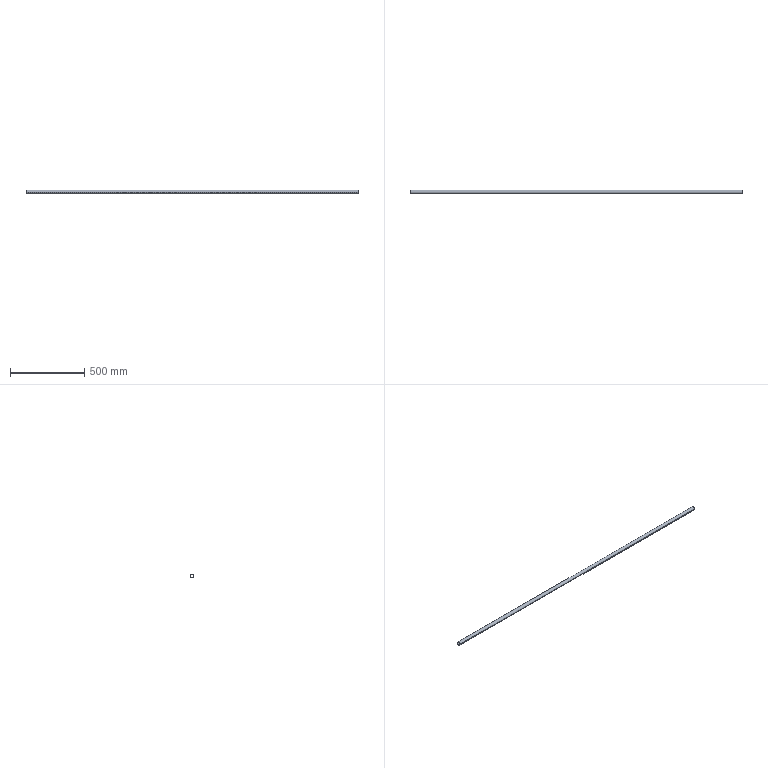Part | STEP file | 电柜通道护栏1栏杆_Default<As Machined> | 1 solid | 6 faces | box 2240 x 25 x 25 mm | volume 248060 mm3 | cylinder 4 | plane 2 | commonest cylinder face diameters 22 x2 25 x2
STEP:
#1=CARTESIAN_POINT('',(0.,0.,0.));
#2=DIRECTION('',(0.,0.,1.));
#3=DIRECTION('',(1.,0.,0.));
#4=AXIS2_PLACEMENT_3D('',#1,#2,#3);
#5=CARTESIAN_POINT('',(1120.,12.5,0.));
#6=VERTEX_POINT('',#5);
#7=CARTESIAN_POINT('',(1120.,-12.5,0.));
#8=VERTEX_POINT('',#7);
#9=CARTESIAN_POINT('',(1120.,0.,0.));
#10=DIRECTION('',(1.,0.,0.));
#11=DIRECTION('',(0.,1.,0.));
#12=AXIS2_PLACEMENT_3D('',#9,#10,#11);
#13=CIRCLE('',#12,12.5);
#14=CARTESIAN_POINT('',(1120.,0.,0.));
#15=DIRECTION('',(-1.,0.,0.));
#16=DIRECTION('',(0.,-1.,0.));
#17=AXIS2_PLACEMENT_3D('',#14,#15,#16);
#18=CYLINDRICAL_SURFACE('',#17,12.5);
#19=CARTESIAN_POINT('',(3.142,0.));
#20=DIRECTION('',(-1.,0.));
#21=VECTOR('',#20,1.);
#22=LINE('',#19,#21);
#23=(GEOMETRIC_REPRESENTATION_CONTEXT(2)PARAMETRIC_REPRESENTATION_CONTEXT()REPRESENTATION_CONTEXT('',''));
#24=DEFINITIONAL_REPRESENTATION('',(#22),#23);
#25=PCURVE('',#18,#24);
#26=CARTESIAN_POINT('',(1120.,0.,0.));
#27=DIRECTION('',(1.,0.,0.));
#28=DIRECTION('',(0.,1.,0.));
#29=AXIS2_PLACEMENT_3D('',#26,#27,#28);
#30=PLANE('',#29);
#31=CARTESIAN_POINT('',(0.,0.));
#32=DIRECTION('',(1.,0.));
#33=AXIS2_PLACEMENT_2D('',#31,#32);
#34=CIRCLE('',#33,12.5);
#35=(GEOMETRIC_REPRESENTATION_CONTEXT(2)PARAMETRIC_REPRESENTATION_CONTEXT()REPRESENTATION_CONTEXT('',''));
#36=DEFINITIONAL_REPRESENTATION('',(#34),#35);
#37=PCURVE('',#30,#36);
#38=SURFACE_CURVE('',#13,(#25,#37),.PCURVE_S1.);
#39=EDGE_CURVE('',#6,#8,#38,.T.);
#40=ORIENTED_EDGE('',*,*,#39,.F.);
#41=CARTESIAN_POINT('',(-1120.,12.5,0.));
#42=VERTEX_POINT('',#41);
#43=CARTESIAN_POINT('',(1120.,12.5,0.));
#44=DIRECTION('',(-1.,0.,0.));
#45=VECTOR('',#44,1.);
#46=LINE('',#43,#45);
#47=CARTESIAN_POINT('',(3.142,0.));
#48=DIRECTION('',(0.,1.));
#49=VECTOR('',#48,1.);
#50=LINE('',#47,#49);
#51=(GEOMETRIC_REPRESENTATION_CONTEXT(2)PARAMETRIC_REPRESENTATION_CONTEXT()REPRESENTATION_CONTEXT('',''));
#52=DEFINITIONAL_REPRESENTATION('',(#50),#51);
#53=PCURVE('',#18,#52);
#54=CARTESIAN_POINT('',(1120.,0.,0.));
#55=DIRECTION('',(-1.,0.,0.));
#56=DIRECTION('',(0.,-1.,0.));
#57=AXIS2_PLACEMENT_3D('',#54,#55,#56);
#58=CYLINDRICAL_SURFACE('',#57,12.5);
#59=CARTESIAN_POINT('',(3.142,0.));
#60=DIRECTION('',(0.,1.));
#61=VECTOR('',#60,1.);
#62=LINE('',#59,#61);
#63=(GEOMETRIC_REPRESENTATION_CONTEXT(2)PARAMETRIC_REPRESENTATION_CONTEXT()REPRESENTATION_CONTEXT('',''));
#64=DEFINITIONAL_REPRESENTATION('',(#62),#63);
#65=PCURVE('',#58,#64);
#66=SURFACE_CURVE('',#46,(#53,#65),.PCURVE_S1.);
#67=EDGE_CURVE('',#6,#42,#66,.T.);
#68=ORIENTED_EDGE('',*,*,#67,.T.);
#69=CARTESIAN_POINT('',(-1120.,-12.5,0.));
#70=VERTEX_POINT('',#69);
#71=CARTESIAN_POINT('',(-1120.,0.,0.));
#72=DIRECTION('',(1.,0.,0.));
#73=DIRECTION('',(0.,1.,0.));
#74=AXIS2_PLACEMENT_3D('',#71,#72,#73);
#75=CIRCLE('',#74,12.5);
#76=CARTESIAN_POINT('',(3.142,2240.));
#77=DIRECTION('',(-1.,0.));
#78=VECTOR('',#77,1.);
#79=LINE('',#76,#78);
#80=(GEOMETRIC_REPRESENTATION_CONTEXT(2)PARAMETRIC_REPRESENTATION_CONTEXT()REPRESENTATION_CONTEXT('',''));
#81=DEFINITIONAL_REPRESENTATION('',(#79),#80);
#82=PCURVE('',#18,#81);
#83=CARTESIAN_POINT('',(-1120.,0.,0.));
#84=DIRECTION('',(1.,0.,0.));
#85=DIRECTION('',(0.,1.,0.));
#86=AXIS2_PLACEMENT_3D('',#83,#84,#85);
#87=PLANE('',#86);
#88=CARTESIAN_POINT('',(0.,0.));
#89=DIRECTION('',(1.,0.));
#90=AXIS2_PLACEMENT_2D('',#88,#89);
#91=CIRCLE('',#90,12.5);
#92=(GEOMETRIC_REPRESENTATION_CONTEXT(2)PARAMETRIC_REPRESENTATION_CONTEXT()REPRESENTATION_CONTEXT('',''));
#93=DEFINITIONAL_REPRESENTATION('',(#91),#92);
#94=PCURVE('',#87,#93);
#95=SURFACE_CURVE('',#75,(#82,#94),.PCURVE_S1.);
#96=EDGE_CURVE('',#42,#70,#95,.T.);
#97=ORIENTED_EDGE('',*,*,#96,.T.);
#98=CARTESIAN_POINT('',(1120.,-12.5,0.));
#99=DIRECTION('',(-1.,0.,0.));
#100=VECTOR('',#99,1.);
#101=LINE('',#98,#100);
#102=CARTESIAN_POINT('',(0.,0.));
#103=DIRECTION('',(0.,1.));
#104=VECTOR('',#103,1.);
#105=LINE('',#102,#104);
#106=(GEOMETRIC_REPRESENTATION_CONTEXT(2)PARAMETRIC_REPRESENTATION_CONTEXT()REPRESENTATION_CONTEXT('',''));
#107=DEFINITIONAL_REPRESENTATION('',(#105),#106);
#108=PCURVE('',#18,#107);
#109=CARTESIAN_POINT('',(6.283,0.));
#110=DIRECTION('',(0.,1.));
#111=VECTOR('',#110,1.);
#112=LINE('',#109,#111);
#113=(GEOMETRIC_REPRESENTATION_CONTEXT(2)PARAMETRIC_REPRESENTATION_CONTEXT()REPRESENTATION_CONTEXT('',''));
#114=DEFINITIONAL_REPRESENTATION('',(#112),#113);
#115=PCURVE('',#58,#114);
#116=SURFACE_CURVE('',#101,(#108,#115),.PCURVE_S1.);
#117=EDGE_CURVE('',#8,#70,#116,.T.);
#118=ORIENTED_EDGE('',*,*,#117,.F.);
#119=EDGE_LOOP('',(#40,#68,#97,#118));
#120=FACE_BOUND('',#119,.T.);
#121=ADVANCED_FACE('',(#120),#18,.T.);
#122=CARTESIAN_POINT('',(1120.,-11.,0.));
#123=VERTEX_POINT('',#122);
#124=CARTESIAN_POINT('',(-1120.,-11.,0.));
#125=VERTEX_POINT('',#124);
#126=CARTESIAN_POINT('',(1120.,-11.,0.));
#127=DIRECTION('',(-1.,0.,0.));
#128=VECTOR('',#127,1.);
#129=LINE('',#126,#128);
#130=CARTESIAN_POINT('',(1120.,0.,0.));
#131=DIRECTION('',(-1.,0.,0.));
#132=DIRECTION('',(0.,-1.,0.));
#133=AXIS2_PLACEMENT_3D('',#130,#131,#132);
#134=CYLINDRICAL_SURFACE('',#133,11.);
#135=CARTESIAN_POINT('',(6.283,0.));
#136=DIRECTION('',(0.,1.));
#137=VECTOR('',#136,1.);
#138=LINE('',#135,#137);
#139=(GEOMETRIC_REPRESENTATION_CONTEXT(2)PARAMETRIC_REPRESENTATION_CONTEXT()REPRESENTATION_CONTEXT('',''));
#140=DEFINITIONAL_REPRESENTATION('',(#138),#139);
#141=PCURVE('',#134,#140);
#142=CARTESIAN_POINT('',(1120.,0.,0.));
#143=DIRECTION('',(-1.,0.,0.));
#144=DIRECTION('',(0.,-1.,0.));
#145=AXIS2_PLACEMENT_3D('',#142,#143,#144);
#146=CYLINDRICAL_SURFACE('',#145,11.);
#147=CARTESIAN_POINT('',(0.,0.));
#148=DIRECTION('',(0.,1.));
#149=VECTOR('',#148,1.);
#150=LINE('',#147,#149);
#151=(GEOMETRIC_REPRESENTATION_CONTEXT(2)PARAMETRIC_REPRESENTATION_CONTEXT()REPRESENTATION_CONTEXT('',''));
#152=DEFINITIONAL_REPRESENTATION('',(#150),#151);
#153=PCURVE('',#146,#152);
#154=SURFACE_CURVE('',#129,(#141,#153),.PCURVE_S1.);
#155=EDGE_CURVE('',#123,#125,#154,.T.);
#156=ORIENTED_EDGE('',*,*,#155,.T.);
#157=CARTESIAN_POINT('',(-1120.,11.,0.));
#158=VERTEX_POINT('',#157);
#159=CARTESIAN_POINT('',(-1120.,0.,0.));
#160=DIRECTION('',(1.,0.,0.));
#161=DIRECTION('',(0.,1.,0.));
#162=AXIS2_PLACEMENT_3D('',#159,#160,#161);
#163=CIRCLE('',#162,11.);
#164=CARTESIAN_POINT('',(9.425,2240.));
#165=DIRECTION('',(-1.,0.));
#166=VECTOR('',#165,1.);
#167=LINE('',#164,#166);
#168=(GEOMETRIC_REPRESENTATION_CONTEXT(2)PARAMETRIC_REPRESENTATION_CONTEXT()REPRESENTATION_CONTEXT('',''));
#169=DEFINITIONAL_REPRESENTATION('',(#167),#168);
#170=PCURVE('',#134,#169);
#171=CARTESIAN_POINT('',(0.,0.));
#172=DIRECTION('',(1.,0.));
#173=AXIS2_PLACEMENT_2D('',#171,#172);
#174=CIRCLE('',#173,11.);
#175=(GEOMETRIC_REPRESENTATION_CONTEXT(2)PARAMETRIC_REPRESENTATION_CONTEXT()REPRESENTATION_CONTEXT('',''));
#176=DEFINITIONAL_REPRESENTATION('',(#174),#175);
#177=PCURVE('',#87,#176);
#178=SURFACE_CURVE('',#163,(#170,#177),.PCURVE_S1.);
#179=EDGE_CURVE('',#125,#158,#178,.T.);
#180=ORIENTED_EDGE('',*,*,#179,.T.);
#181=CARTESIAN_POINT('',(1120.,11.,0.));
#182=VERTEX_POINT('',#181);
#183=CARTESIAN_POINT('',(1120.,11.,0.));
#184=DIRECTION('',(-1.,0.,0.));
#185=VECTOR('',#184,1.);
#186=LINE('',#183,#185);
#187=CARTESIAN_POINT('',(3.142,0.));
#188=DIRECTION('',(0.,1.));
#189=VECTOR('',#188,1.);
#190=LINE('',#187,#189);
#191=(GEOMETRIC_REPRESENTATION_CONTEXT(2)PARAMETRIC_REPRESENTATION_CONTEXT()REPRESENTATION_CONTEXT('',''));
#192=DEFINITIONAL_REPRESENTATION('',(#190),#191);
#193=PCURVE('',#134,#192);
#194=CARTESIAN_POINT('',(3.142,0.));
#195=DIRECTION('',(0.,1.));
#196=VECTOR('',#195,1.);
#197=LINE('',#194,#196);
#198=(GEOMETRIC_REPRESENTATION_CONTEXT(2)PARAMETRIC_REPRESENTATION_CONTEXT()REPRESENTATION_CONTEXT('',''));
#199=DEFINITIONAL_REPRESENTATION('',(#197),#198);
#200=PCURVE('',#146,#199);
#201=SURFACE_CURVE('',#186,(#193,#200),.PCURVE_S1.);
#202=EDGE_CURVE('',#182,#158,#201,.T.);
#203=ORIENTED_EDGE('',*,*,#202,.F.);
#204=CARTESIAN_POINT('',(1120.,0.,0.));
#205=DIRECTION('',(1.,0.,0.));
#206=DIRECTION('',(0.,1.,0.));
#207=AXIS2_PLACEMENT_3D('',#204,#205,#206);
#208=CIRCLE('',#207,11.);
#209=CARTESIAN_POINT('',(9.425,0.));
#210=DIRECTION('',(-1.,0.));
#211=VECTOR('',#210,1.);
#212=LINE('',#209,#211);
#213=(GEOMETRIC_REPRESENTATION_CONTEXT(2)PARAMETRIC_REPRESENTATION_CONTEXT()REPRESENTATION_CONTEXT('',''));
#214=DEFINITIONAL_REPRESENTATION('',(#212),#213);
#215=PCURVE('',#134,#214);
#216=CARTESIAN_POINT('',(0.,0.));
#217=DIRECTION('',(1.,0.));
#218=AXIS2_PLACEMENT_2D('',#216,#217);
#219=CIRCLE('',#218,11.);
#220=(GEOMETRIC_REPRESENTATION_CONTEXT(2)PARAMETRIC_REPRESENTATION_CONTEXT()REPRESENTATION_CONTEXT('',''));
#221=DEFINITIONAL_REPRESENTATION('',(#219),#220);
#222=PCURVE('',#30,#221);
#223=SURFACE_CURVE('',#208,(#215,#222),.PCURVE_S1.);
#224=EDGE_CURVE('',#123,#182,#223,.T.);
#225=ORIENTED_EDGE('',*,*,#224,.F.);
#226=EDGE_LOOP('',(#156,#180,#203,#225));
#227=FACE_BOUND('',#226,.F.);
#228=ADVANCED_FACE('',(#227),#134,.F.);
#229=CARTESIAN_POINT('',(-1120.,0.,0.));
#230=DIRECTION('',(1.,0.,0.));
#231=DIRECTION('',(0.,1.,0.));
#232=AXIS2_PLACEMENT_3D('',#229,#230,#231);
#233=CIRCLE('',#232,11.);
#234=CARTESIAN_POINT('',(3.142,2240.));
#235=DIRECTION('',(-1.,0.));
#236=VECTOR('',#235,1.);
#237=LINE('',#234,#236);
#238=(GEOMETRIC_REPRESENTATION_CONTEXT(2)PARAMETRIC_REPRESENTATION_CONTEXT()REPRESENTATION_CONTEXT('',''));
#239=DEFINITIONAL_REPRESENTATION('',(#237),#238);
#240=PCURVE('',#146,#239);
#241=CARTESIAN_POINT('',(0.,0.));
#242=DIRECTION('',(1.,0.));
#243=AXIS2_PLACEMENT_2D('',#241,#242);
#244=CIRCLE('',#243,11.);
#245=(GEOMETRIC_REPRESENTATION_CONTEXT(2)PARAMETRIC_REPRESENTATION_CONTEXT()REPRESENTATION_CONTEXT('',''));
#246=DEFINITIONAL_REPRESENTATION('',(#244),#245);
#247=PCURVE('',#87,#246);
#248=SURFACE_CURVE('',#233,(#240,#247),.PCURVE_S1.);
#249=EDGE_CURVE('',#158,#125,#248,.T.);
#250=ORIENTED_EDGE('',*,*,#249,.T.);
#251=ORIENTED_EDGE('',*,*,#155,.F.);
#252=CARTESIAN_POINT('',(1120.,0.,0.));
#253=DIRECTION('',(1.,0.,0.));
#254=DIRECTION('',(0.,1.,0.));
#255=AXIS2_PLACEMENT_3D('',#252,#253,#254);
#256=CIRCLE('',#255,11.);
#257=CARTESIAN_POINT('',(3.142,0.));
#258=DIRECTION('',(-1.,0.));
#259=VECTOR('',#258,1.);
#260=LINE('',#257,#259);
#261=(GEOMETRIC_REPRESENTATION_CONTEXT(2)PARAMETRIC_REPRESENTATION_CONTEXT()REPRESENTATION_CONTEXT('',''));
#262=DEFINITIONAL_REPRESENTATION('',(#260),#261);
#263=PCURVE('',#146,#262);
#264=CARTESIAN_POINT('',(0.,0.));
#265=DIRECTION('',(1.,0.));
#266=AXIS2_PLACEMENT_2D('',#264,#265);
#267=CIRCLE('',#266,11.);
#268=(GEOMETRIC_REPRESENTATION_CONTEXT(2)PARAMETRIC_REPRESENTATION_CONTEXT()REPRESENTATION_CONTEXT('',''));
#269=DEFINITIONAL_REPRESENTATION('',(#267),#268);
#270=PCURVE('',#30,#269);
#271=SURFACE_CURVE('',#256,(#263,#270),.PCURVE_S1.);
#272=EDGE_CURVE('',#182,#123,#271,.T.);
#273=ORIENTED_EDGE('',*,*,#272,.F.);
#274=ORIENTED_EDGE('',*,*,#202,.T.);
#275=EDGE_LOOP('',(#250,#251,#273,#274));
#276=FACE_BOUND('',#275,.F.);
#277=ADVANCED_FACE('',(#276),#146,.F.);
#278=ORIENTED_EDGE('',*,*,#67,.F.);
#279=CARTESIAN_POINT('',(1120.,0.,0.));
#280=DIRECTION('',(1.,0.,0.));
#281=DIRECTION('',(0.,1.,0.));
#282=AXIS2_PLACEMENT_3D('',#279,#280,#281);
#283=CIRCLE('',#282,12.5);
#284=CARTESIAN_POINT('',(9.425,0.));
#285=DIRECTION('',(-1.,0.));
#286=VECTOR('',#285,1.);
#287=LINE('',#284,#286);
#288=(GEOMETRIC_REPRESENTATION_CONTEXT(2)PARAMETRIC_REPRESENTATION_CONTEXT()REPRESENTATION_CONTEXT('',''));
#289=DEFINITIONAL_REPRESENTATION('',(#287),#288);
#290=PCURVE('',#58,#289);
#291=CARTESIAN_POINT('',(0.,0.));
#292=DIRECTION('',(1.,0.));
#293=AXIS2_PLACEMENT_2D('',#291,#292);
#294=CIRCLE('',#293,12.5);
#295=(GEOMETRIC_REPRESENTATION_CONTEXT(2)PARAMETRIC_REPRESENTATION_CONTEXT()REPRESENTATION_CONTEXT('',''));
#296=DEFINITIONAL_REPRESENTATION('',(#294),#295);
#297=PCURVE('',#30,#296);
#298=SURFACE_CURVE('',#283,(#290,#297),.PCURVE_S1.);
#299=EDGE_CURVE('',#8,#6,#298,.T.);
#300=ORIENTED_EDGE('',*,*,#299,.F.);
#301=ORIENTED_EDGE('',*,*,#117,.T.);
#302=CARTESIAN_POINT('',(-1120.,0.,0.));
#303=DIRECTION('',(1.,0.,0.));
#304=DIRECTION('',(0.,1.,0.));
#305=AXIS2_PLACEMENT_3D('',#302,#303,#304);
#306=CIRCLE('',#305,12.5);
#307=CARTESIAN_POINT('',(9.425,2240.));
#308=DIRECTION('',(-1.,0.));
#309=VECTOR('',#308,1.);
#310=LINE('',#307,#309);
#311=(GEOMETRIC_REPRESENTATION_CONTEXT(2)PARAMETRIC_REPRESENTATION_CONTEXT()REPRESENTATION_CONTEXT('',''));
#312=DEFINITIONAL_REPRESENTATION('',(#310),#311);
#313=PCURVE('',#58,#312);
#314=CARTESIAN_POINT('',(0.,0.));
#315=DIRECTION('',(1.,0.));
#316=AXIS2_PLACEMENT_2D('',#314,#315);
#317=CIRCLE('',#316,12.5);
#318=(GEOMETRIC_REPRESENTATION_CONTEXT(2)PARAMETRIC_REPRESENTATION_CONTEXT()REPRESENTATION_CONTEXT('',''));
#319=DEFINITIONAL_REPRESENTATION('',(#317),#318);
#320=PCURVE('',#87,#319);
#321=SURFACE_CURVE('',#306,(#313,#320),.PCURVE_S1.);
#322=EDGE_CURVE('',#70,#42,#321,.T.);
#323=ORIENTED_EDGE('',*,*,#322,.T.);
#324=EDGE_LOOP('',(#278,#300,#301,#323));
#325=FACE_BOUND('',#324,.T.);
#326=ADVANCED_FACE('',(#325),#58,.T.);
#327=ORIENTED_EDGE('',*,*,#224,.F.);
#328=ORIENTED_EDGE('',*,*,#272,.F.);
#329=EDGE_LOOP('',(#327,#328));
#330=FACE_BOUND('',#329,.T.);
#331=ORIENTED_EDGE('',*,*,#299,.T.);
#332=ORIENTED_EDGE('',*,*,#39,.T.);
#333=EDGE_LOOP('',(#331,#332));
#334=FACE_BOUND('',#333,.T.);
#335=ADVANCED_FACE('',(#330,#334),#30,.T.);
#336=ORIENTED_EDGE('',*,*,#179,.T.);
#337=ORIENTED_EDGE('',*,*,#249,.T.);
#338=EDGE_LOOP('',(#336,#337));
#339=FACE_BOUND('',#338,.T.);
#340=ORIENTED_EDGE('',*,*,#322,.F.);
#341=ORIENTED_EDGE('',*,*,#96,.F.);
#342=EDGE_LOOP('',(#340,#341));
#343=FACE_BOUND('',#342,.T.);
#344=ADVANCED_FACE('',(#339,#343),#87,.F.);
#345=CLOSED_SHELL('',(#121,#228,#277,#326,#335,#344));
#346=MANIFOLD_SOLID_BREP('',#345);
#347=(LENGTH_UNIT()NAMED_UNIT(*)SI_UNIT(.MILLI.,.METRE.));
#348=UNCERTAINTY_MEASURE_WITH_UNIT(LENGTH_MEASURE(0.0000001),#347,'','');
#349=(NAMED_UNIT(*)PLANE_ANGLE_UNIT()SI_UNIT($,.RADIAN.));
#350=(NAMED_UNIT(*)SI_UNIT($,.STERADIAN.)SOLID_ANGLE_UNIT());
#351=(GEOMETRIC_REPRESENTATION_CONTEXT(3)GLOBAL_UNCERTAINTY_ASSIGNED_CONTEXT((#348))GLOBAL_UNIT_ASSIGNED_CONTEXT((#347,#349,#350))REPRESENTATION_CONTEXT('',''));
#352=ADVANCED_BREP_SHAPE_REPRESENTATION('',(#4,#346),#351);